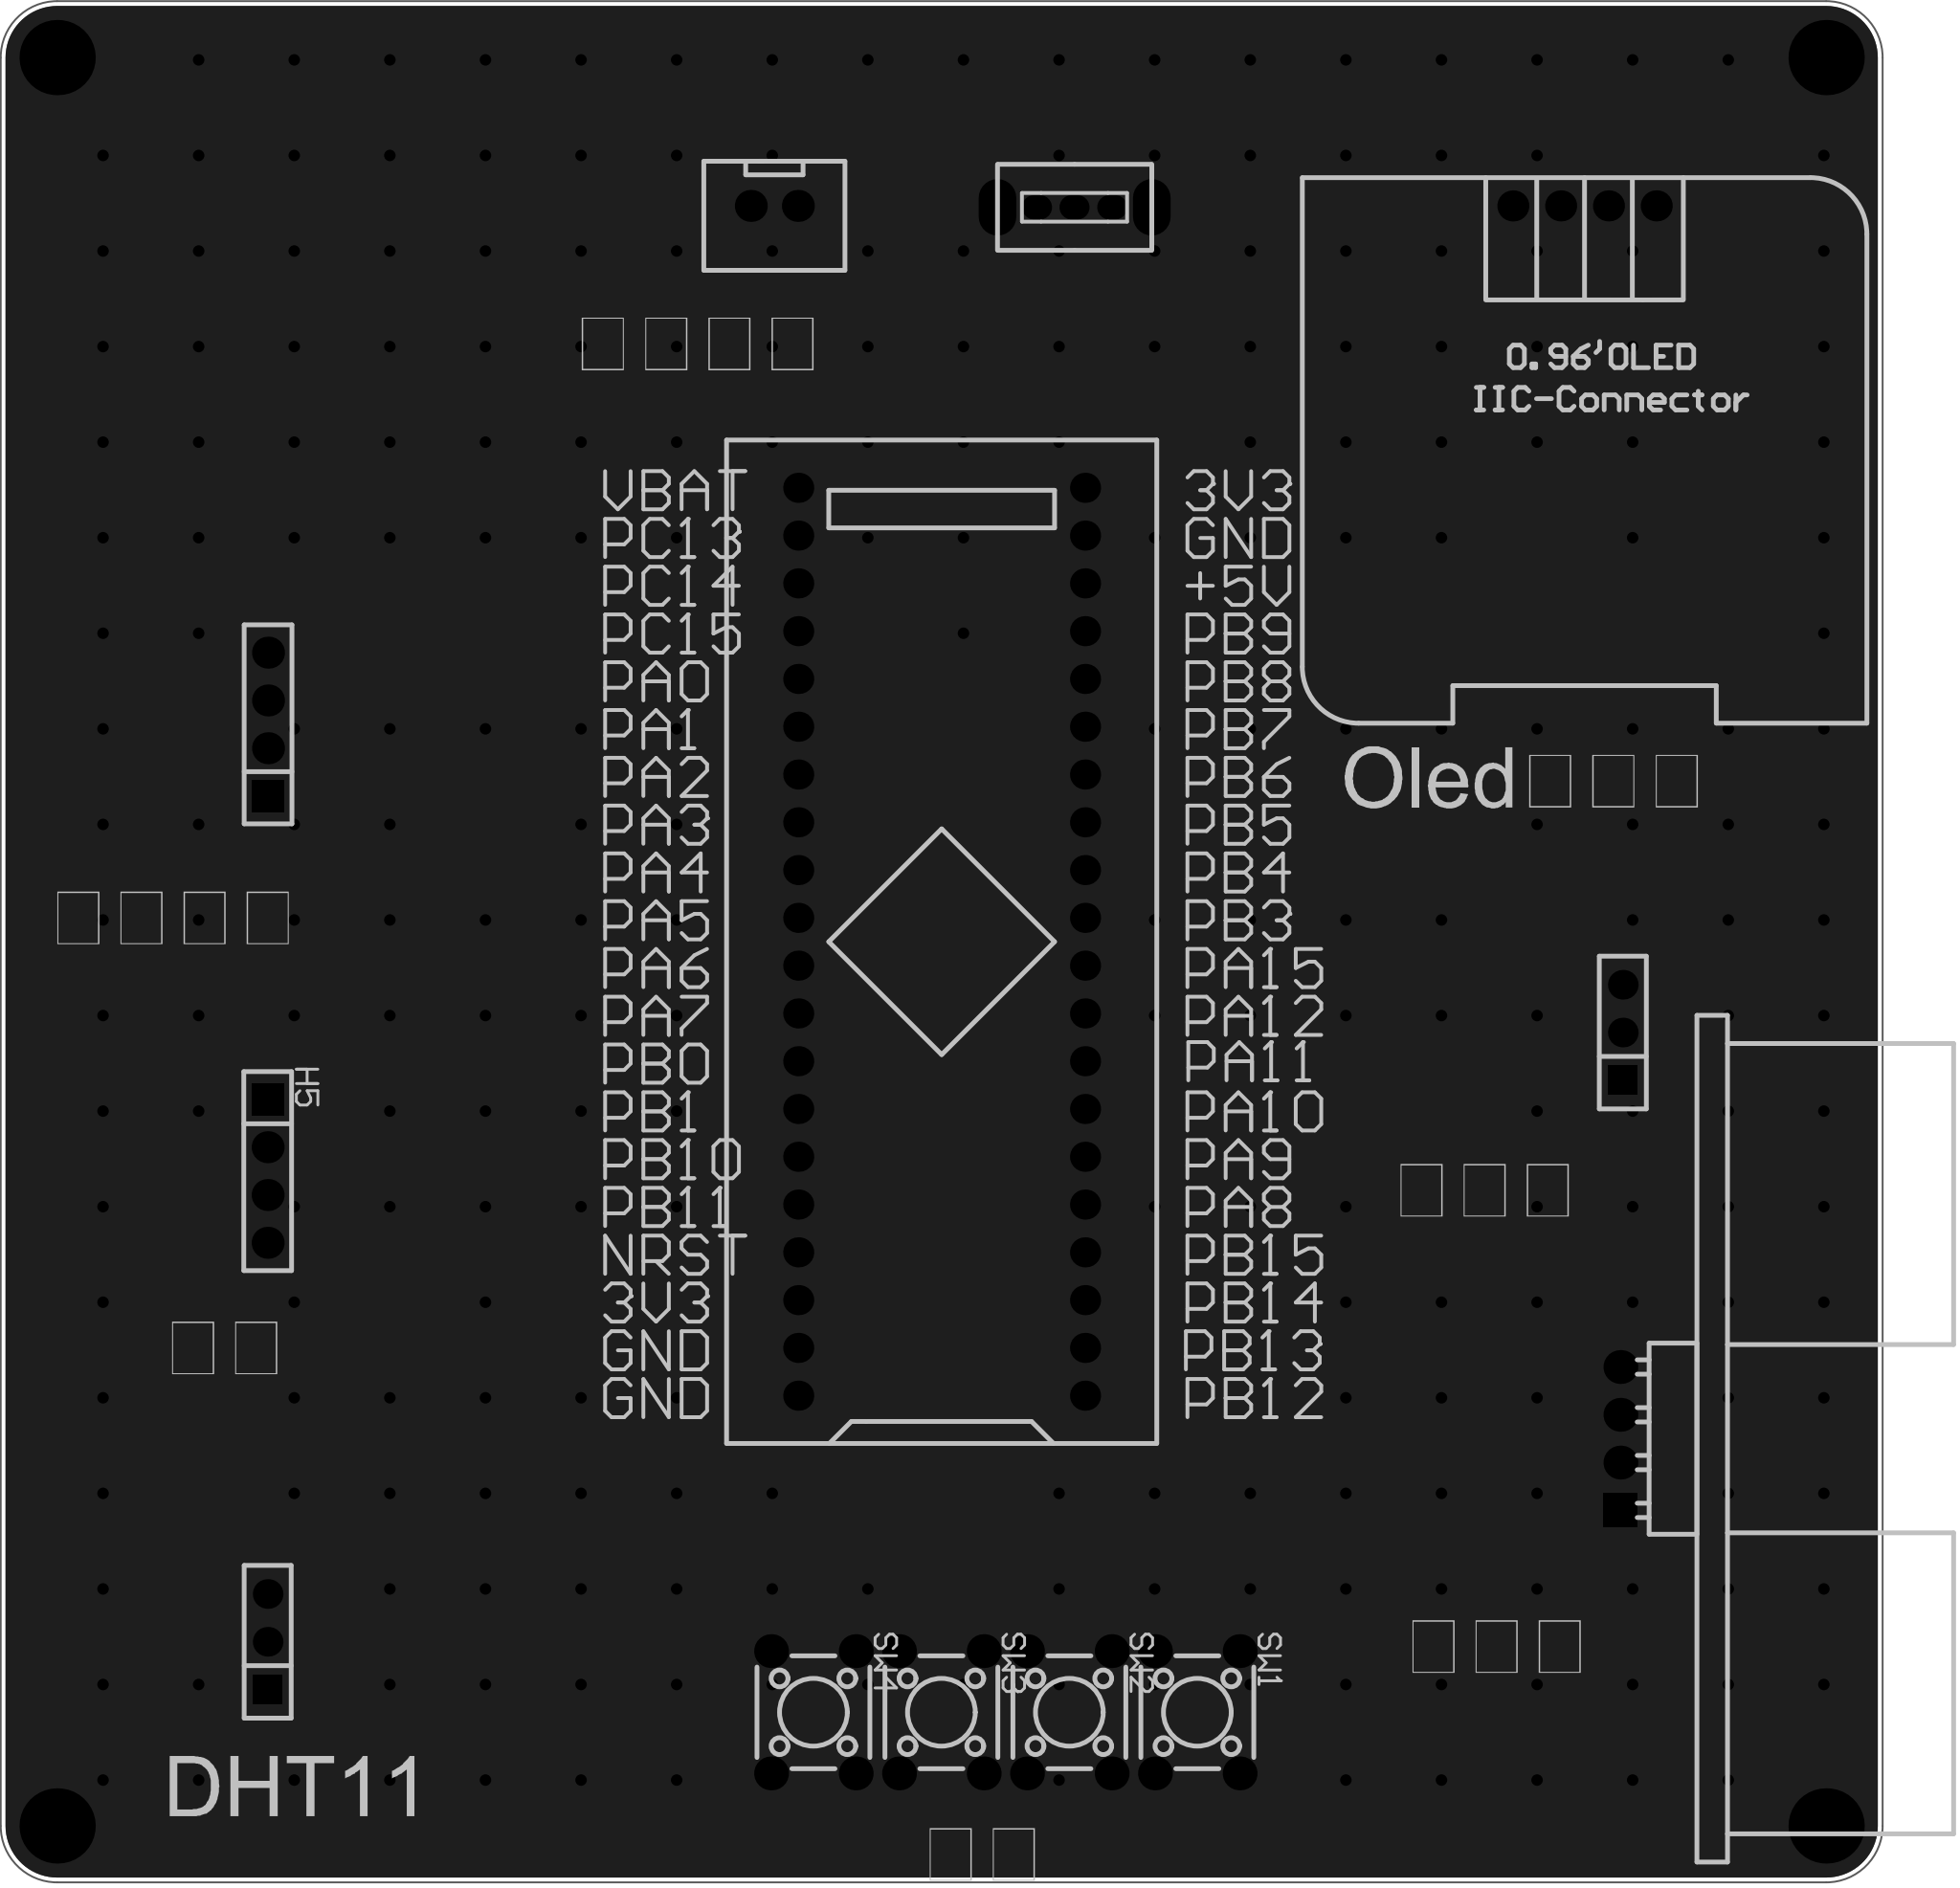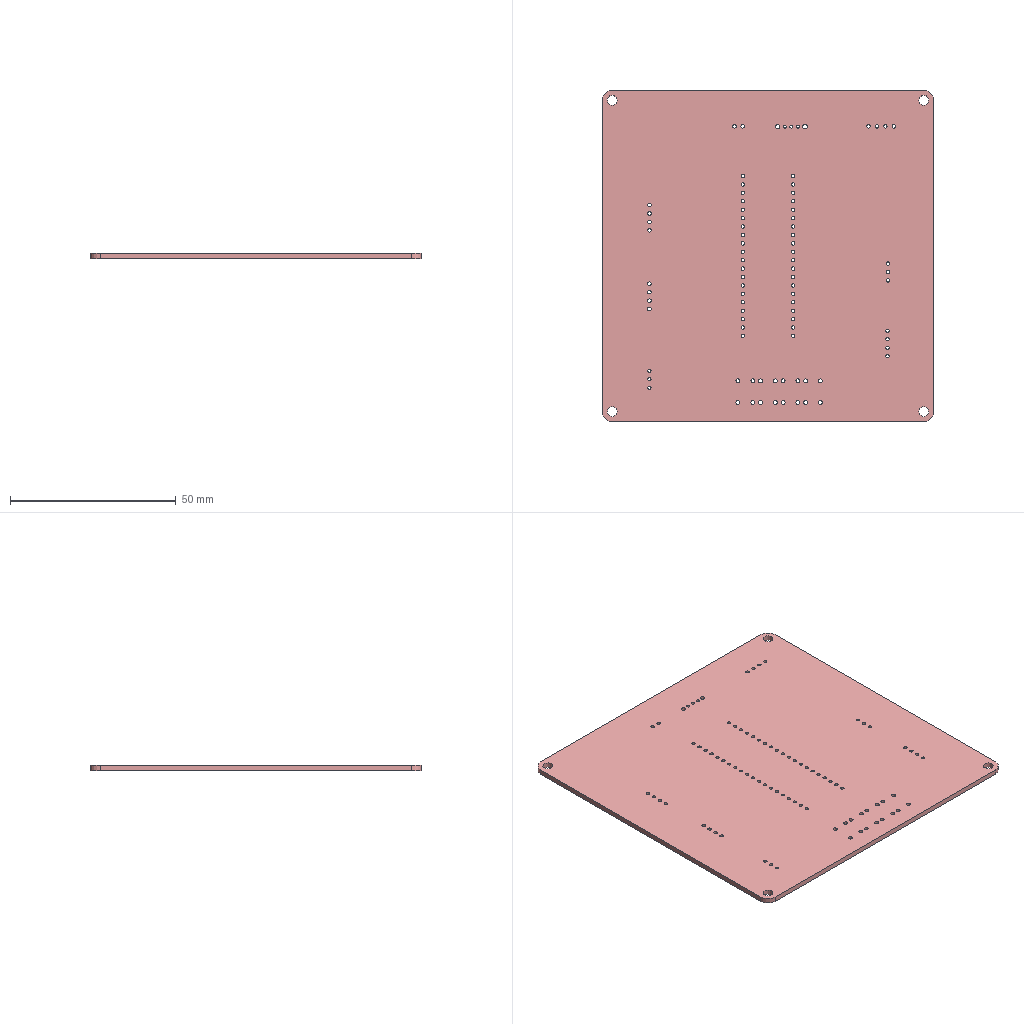Circuit board layout | Altium Designer | box 100 x 100 x 1.6 mm
Layer stack:
# Altium Designer layer stack of  (unit mm; dielectric type: 0 none, 1 core, 2 prepreg, 3 surface material)
index,name,kind,layer,copper_thickness_mm,dielectric_type,dielectric_thickness_mm,dielectric_material,dielectric_constant
0,Top Paste Mask Layer,other,,,,,,
1,Top Silkscreen Layer,other,,,,,,
2,Top Solder Mask Layer,dielectric,,,3,0.01,,3.3
3,Top Layer,copper,Top Layer,0.035,,,,
4,Dielectric1,dielectric,,,3,1.51,FR4,4.5
5,Bottom Layer,copper,Bottom Layer,0.035,,,,
6,Bottom Solder Mask Layer,dielectric,,,3,0.01,,3.3
7,Bottom Silkscreen Layer,other,,,,,,
8,Bottom Paste Mask Layer,other,,,,,,
# drill layer pairs: low layer,high layer
drill_pair,Top Layer,Bottom Layer
Part placement:
Designator,Comment,Layer,Footprint,Center-X(mm),Center-Y(mm),Rotation
U1,STM32F103C8T6-Card,TopLayer,CONN-TH_L53.3-W22.9_STM32F103C8T6-CARD,141.351,130.937,90
OLED1,,TopLayer,0.96OLED_4P,175.514,170.053,0
SW1,,TopLayer,SW-TH_4P-L6.0-W6.0-P4.50-LS6.5,154.936,89.979,270
SW2,,TopLayer,SW-TH_4P-L6.0-W6.0-P4.50-LS6.5,148.136,89.979,270
SW3,,TopLayer,SW-TH_4P-L6.0-W6.0-P4.50-LS6.5,141.337,89.979,270
SW4,,TopLayer,SW-TH_4P-L6.0-W6.0-P4.50-LS6.5,134.537,89.979,270
CN4,XH2.54*2P_直插,TopLayer,CONN-TH_2P-P2.50-XH2.54-2P,132.461,170.053,0
SW5,,TopLayer,拨动开关,148.417,169.978,0
H1,,TopLayer,HDR-TH_3P-P2.54-V-F,177.546,126.111,90
H3,,TopLayer,HDR-TH_3P-P2.54-V-F,105.537,93.726,90
H4,,TopLayer,HDR-TH_4P-P2.54-V-F,105.557,142.494,90
H5,,TopLayer,HDR-TH_4P-P2.54-V-F,105.537,118.745,270
U2,HC-SR04,TopLayer,TH_HC-SR04V,177.419,104.521,90
Pad and via stacks:
# Altium Designer via and pad stacks of  (unit mm). Each distinct definition once, with the count of objects using it.
# via: kind,start_layer,end_layer,hole_mm,diameter_mm,mode(0 simple;1 top-mid-bottom;2 full stack),diameter_per_layer,count,example_net
# pad: kind,layer,hole_mm,hole_type(0 round;1 square;2 slot),plating,top_size,top_shape(1 round;2 rect;3 octagon;9 rounded rect),mid_size,bottom_size,mode,footprint,size_per_layer,count,example
pad,Multi-Layer,3,0,plated,4x4,1,4x4,4x4,0,,,4,1
pad,Multi-Layer,1,0,plated,1.6x1.6,1,1.6x1.6,1.6x1.6,0,CONN-TH_L53.3-W22.9_STM32F103C8T6-CARD,,40,U1.1
pad,Multi-Layer,1,0,plated,1.65x1.65,1,1.65x1.65,1.65x1.65,0,0.96OLED_4P,,4,OLED1.4
pad,Multi-Layer,1.2,0,plated,1.8x1.8,1,1.8x1.8,1.8x1.8,0,SW-TH_4P-L6.0-W6.0-P4.50-LS6.5,,16,SW1.1
pad,Multi-Layer,1.05,0,plated,1.7x1.7,1,1.7x1.7,1.7x1.7,0,CONN-TH_2P-P2.50-XH2.54-2P,,2,CN4.2
pad,Multi-Layer,0.8992,0,plated,1.6x1.3,1,1.6x1.3,1.6x1.3,0,\u00B2\u00A6\u00B6\u00AF\u00BF\u00AA\u00B9\u00D8,,3,SW5.1
pad,Multi-Layer,1.3,0,plated,3x1.999,1,3x1.999,3x1.999,0,\u00B2\u00A6\u00B6\u00AF\u00BF\u00AA\u00B9\u00D8,,2,SW5.4
pad,Multi-Layer,1.02,0,plated,1.575x1.575,1,1.575x1.575,1.575x1.575,0,HDR-TH_3P-P2.54-V-F,,4,H1.3
pad,Multi-Layer,1.02,0,plated,1.575x1.575,2,1.575x1.575,1.575x1.575,0,HDR-TH_3P-P2.54-V-F,,2,H1.1
pad,Multi-Layer,1.1,0,plated,1.7x1.7,2,1.7x1.7,1.7x1.7,0,HDR-TH_4P-P2.54-V-F,,2,H4.1
pad,Multi-Layer,1.1,0,plated,1.7x1.7,1,1.7x1.7,1.7x1.7,0,HDR-TH_4P-P2.54-V-F,,6,H4.2
pad,Multi-Layer,1.001,0,plated,1.8x1.8,1,1.8x1.8,1.8x1.8,0,TH_HC-SR04V,,3,U2.4
pad,Multi-Layer,1.001,0,plated,1.8x1.8,2,1.8x1.8,1.8x1.8,0,TH_HC-SR04V,,1,U2.1
via,Top Layer,Bottom Layer,0.3048,0.61,0,,261,GND
Copper pours:
name,layer,net,type(0 solid;1 hatched;2 none)
Bottom Layer-GND,Bottom Layer,GND,0
Top Layer-GND,Top Layer,GND,0